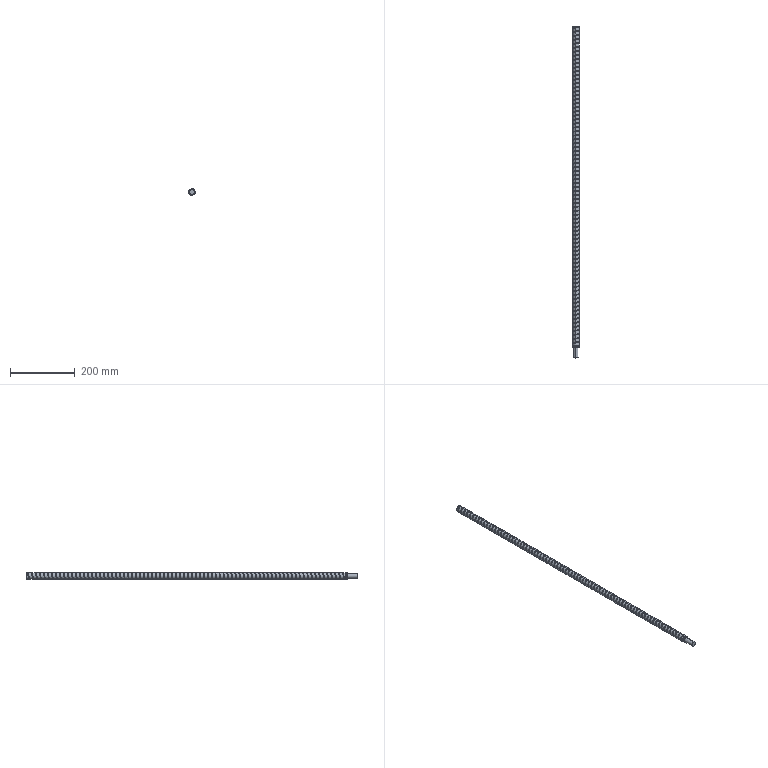Part | SolidWorks | features Revolution 2, Helix 1, MoveFace 1, SweepCut 1 | 1 solid | 185 faces | box 20 x 1028 x 20 mm | volume 299367 mm3 | cylinder 173 | plane 10 | spline 2 | commonest cylinder face diameters 20 x162 15 x8 19 x3